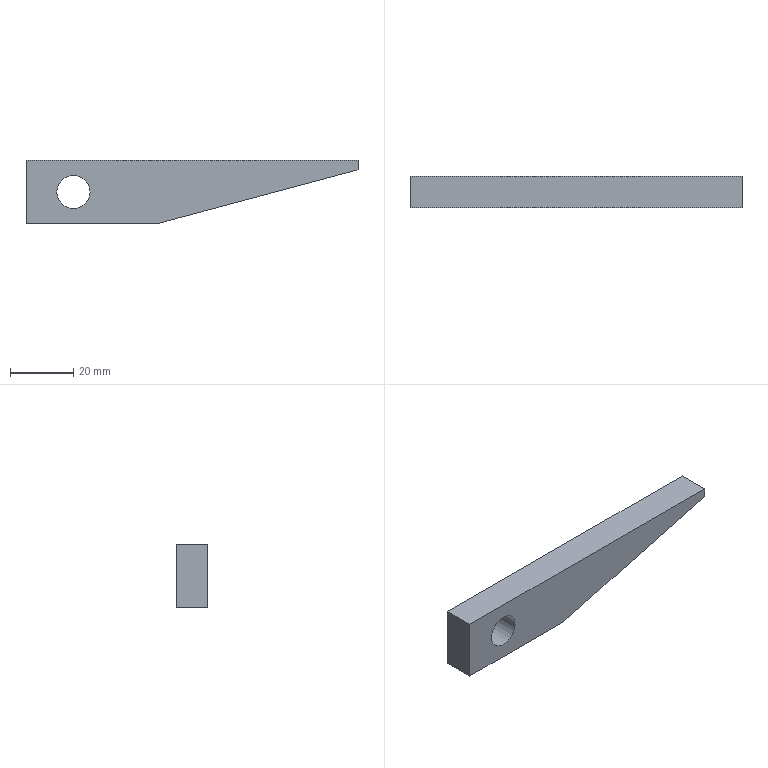Part | NX | features solid 2 | 1 solid | 8 faces | box 105 x 10 x 20 mm | volume 14741 mm3 | plane 7 | cylinder 1 | commonest cylinder face diameters 10.5 x1
STEP:
#1=CARTESIAN_POINT('',(-925.,90.,-134.));
#2=VERTEX_POINT('',#1);
#3=CARTESIAN_POINT('',(-883.445,90.,-134.));
#4=VERTEX_POINT('',#3);
#5=CARTESIAN_POINT('',(-925.,90.,-134.));
#6=DIRECTION('',(1.,0.,0.));
#7=VECTOR('',#6,1000.);
#8=LINE('',#5,#7);
#9=EDGE_CURVE('',#2,#4,#8,.T.);
#10=ORIENTED_EDGE('',*,*,#9,.T.);
#11=CARTESIAN_POINT('',(-883.445,80.,-134.));
#12=VERTEX_POINT('',#11);
#13=CARTESIAN_POINT('',(-883.445,90.,-134.));
#14=DIRECTION('',(0.,-1.,0.));
#15=VECTOR('',#14,1000.);
#16=LINE('',#13,#15);
#17=EDGE_CURVE('',#4,#12,#16,.T.);
#18=ORIENTED_EDGE('',*,*,#17,.T.);
#19=CARTESIAN_POINT('',(-925.,80.,-134.));
#20=VERTEX_POINT('',#19);
#21=CARTESIAN_POINT('',(-925.,80.,-134.));
#22=DIRECTION('',(1.,0.,0.));
#23=VECTOR('',#22,1000.);
#24=LINE('',#21,#23);
#25=EDGE_CURVE('',#20,#12,#24,.T.);
#26=ORIENTED_EDGE('',*,*,#25,.F.);
#27=CARTESIAN_POINT('',(-925.,90.,-134.));
#28=DIRECTION('',(0.,-1.,0.));
#29=VECTOR('',#28,1000.);
#30=LINE('',#27,#29);
#31=EDGE_CURVE('',#2,#20,#30,.T.);
#32=ORIENTED_EDGE('',*,*,#31,.F.);
#33=EDGE_LOOP('',(#10,#18,#26,#32));
#34=FACE_BOUND('',#33,.T.);
#35=CARTESIAN_POINT('',(-925.,90.,-134.));
#36=DIRECTION('',(0.,0.,-1.));
#37=DIRECTION('',(-1.,0.,0.));
#38=AXIS2_PLACEMENT_3D('',#35,#36,#37);
#39=PLANE('',#38);
#40=ADVANCED_FACE('',(#34),#39,.T.);
#41=CARTESIAN_POINT('',(-820.,80.,-117.));
#42=VERTEX_POINT('',#41);
#43=CARTESIAN_POINT('',(-820.,80.,-114.));
#44=VERTEX_POINT('',#43);
#45=CARTESIAN_POINT('',(-820.,80.,-134.));
#46=DIRECTION('',(0.,0.,1.));
#47=VECTOR('',#46,1000.);
#48=LINE('',#45,#47);
#49=EDGE_CURVE('',#42,#44,#48,.T.);
#50=ORIENTED_EDGE('',*,*,#49,.F.);
#51=CARTESIAN_POINT('',(-820.,90.,-117.));
#52=VERTEX_POINT('',#51);
#53=CARTESIAN_POINT('',(-820.,90.,-117.));
#54=DIRECTION('',(0.,1.,0.));
#55=VECTOR('',#54,1000.);
#56=LINE('',#53,#55);
#57=EDGE_CURVE('',#42,#52,#56,.T.);
#58=ORIENTED_EDGE('',*,*,#57,.T.);
#59=CARTESIAN_POINT('',(-820.,90.,-114.));
#60=VERTEX_POINT('',#59);
#61=CARTESIAN_POINT('',(-820.,90.,-134.));
#62=DIRECTION('',(0.,0.,1.));
#63=VECTOR('',#62,1000.);
#64=LINE('',#61,#63);
#65=EDGE_CURVE('',#52,#60,#64,.T.);
#66=ORIENTED_EDGE('',*,*,#65,.T.);
#67=CARTESIAN_POINT('',(-820.,90.,-114.));
#68=DIRECTION('',(0.,-1.,0.));
#69=VECTOR('',#68,1000.);
#70=LINE('',#67,#69);
#71=EDGE_CURVE('',#60,#44,#70,.T.);
#72=ORIENTED_EDGE('',*,*,#71,.T.);
#73=EDGE_LOOP('',(#50,#58,#66,#72));
#74=FACE_BOUND('',#73,.T.);
#75=CARTESIAN_POINT('',(-820.,90.,-134.));
#76=DIRECTION('',(1.,0.,0.));
#77=DIRECTION('',(0.,0.,-1.));
#78=AXIS2_PLACEMENT_3D('',#75,#76,#77);
#79=PLANE('',#78);
#80=ADVANCED_FACE('',(#74),#79,.T.);
#81=CARTESIAN_POINT('',(-925.,80.,-114.));
#82=VERTEX_POINT('',#81);
#83=CARTESIAN_POINT('',(-820.,80.,-114.));
#84=DIRECTION('',(-1.,0.,0.));
#85=VECTOR('',#84,1000.);
#86=LINE('',#83,#85);
#87=EDGE_CURVE('',#44,#82,#86,.T.);
#88=ORIENTED_EDGE('',*,*,#87,.F.);
#89=ORIENTED_EDGE('',*,*,#71,.F.);
#90=CARTESIAN_POINT('',(-925.,90.,-114.));
#91=VERTEX_POINT('',#90);
#92=CARTESIAN_POINT('',(-820.,90.,-114.));
#93=DIRECTION('',(-1.,0.,0.));
#94=VECTOR('',#93,1000.);
#95=LINE('',#92,#94);
#96=EDGE_CURVE('',#60,#91,#95,.T.);
#97=ORIENTED_EDGE('',*,*,#96,.T.);
#98=CARTESIAN_POINT('',(-925.,90.,-114.));
#99=DIRECTION('',(0.,-1.,0.));
#100=VECTOR('',#99,1000.);
#101=LINE('',#98,#100);
#102=EDGE_CURVE('',#91,#82,#101,.T.);
#103=ORIENTED_EDGE('',*,*,#102,.T.);
#104=EDGE_LOOP('',(#88,#89,#97,#103));
#105=FACE_BOUND('',#104,.T.);
#106=CARTESIAN_POINT('',(-820.,90.,-114.));
#107=DIRECTION('',(0.,0.,1.));
#108=DIRECTION('',(0.,1.,0.));
#109=AXIS2_PLACEMENT_3D('',#106,#107,#108);
#110=PLANE('',#109);
#111=ADVANCED_FACE('',(#105),#110,.T.);
#112=CARTESIAN_POINT('',(-925.,80.,-114.));
#113=DIRECTION('',(0.,0.,-1.));
#114=VECTOR('',#113,1000.);
#115=LINE('',#112,#114);
#116=EDGE_CURVE('',#82,#20,#115,.T.);
#117=ORIENTED_EDGE('',*,*,#116,.F.);
#118=ORIENTED_EDGE('',*,*,#102,.F.);
#119=CARTESIAN_POINT('',(-925.,90.,-114.));
#120=DIRECTION('',(0.,0.,-1.));
#121=VECTOR('',#120,1000.);
#122=LINE('',#119,#121);
#123=EDGE_CURVE('',#91,#2,#122,.T.);
#124=ORIENTED_EDGE('',*,*,#123,.T.);
#125=ORIENTED_EDGE('',*,*,#31,.T.);
#126=EDGE_LOOP('',(#117,#118,#124,#125));
#127=FACE_BOUND('',#126,.T.);
#128=CARTESIAN_POINT('',(-925.,90.,-114.));
#129=DIRECTION('',(-1.,0.,0.));
#130=DIRECTION('',(0.,0.,1.));
#131=AXIS2_PLACEMENT_3D('',#128,#129,#130);
#132=PLANE('',#131);
#133=ADVANCED_FACE('',(#127),#132,.T.);
#134=CARTESIAN_POINT('',(-915.25,90.,-124.));
#135=VERTEX_POINT('',#134);
#136=CARTESIAN_POINT('',(-910.,90.,-124.));
#137=DIRECTION('',(0.,1.,0.));
#138=DIRECTION('',(-1.,0.,0.));
#139=AXIS2_PLACEMENT_3D('',#136,#137,#138);
#140=CIRCLE('',#139,5.25);
#141=EDGE_CURVE('',#135,#135,#140,.T.);
#142=ORIENTED_EDGE('',*,*,#141,.T.);
#143=EDGE_LOOP('',(#142));
#144=FACE_BOUND('',#143,.T.);
#145=CARTESIAN_POINT('',(-915.25,80.,-124.));
#146=VERTEX_POINT('',#145);
#147=CARTESIAN_POINT('',(-910.,80.,-124.));
#148=DIRECTION('',(0.,1.,0.));
#149=DIRECTION('',(-1.,0.,0.));
#150=AXIS2_PLACEMENT_3D('',#147,#148,#149);
#151=CIRCLE('',#150,5.25);
#152=EDGE_CURVE('',#146,#146,#151,.T.);
#153=ORIENTED_EDGE('',*,*,#152,.F.);
#154=EDGE_LOOP('',(#153));
#155=FACE_BOUND('',#154,.T.);
#156=CARTESIAN_POINT('',(-910.,90.,-124.));
#157=DIRECTION('',(0.,-1.,0.));
#158=DIRECTION('',(0.,0.,1.));
#159=AXIS2_PLACEMENT_3D('',#156,#157,#158);
#160=CYLINDRICAL_SURFACE('',#159,5.25);
#161=ADVANCED_FACE('',(#144,#155),#160,.F.);
#162=ORIENTED_EDGE('',*,*,#65,.F.);
#163=CARTESIAN_POINT('',(-883.445,90.,-134.));
#164=DIRECTION('',(0.9659,0.,0.2588));
#165=VECTOR('',#164,1000.);
#166=LINE('',#163,#165);
#167=EDGE_CURVE('',#52,#4,#166,.F.);
#168=ORIENTED_EDGE('',*,*,#167,.T.);
#169=ORIENTED_EDGE('',*,*,#9,.F.);
#170=ORIENTED_EDGE('',*,*,#123,.F.);
#171=ORIENTED_EDGE('',*,*,#96,.F.);
#172=EDGE_LOOP('',(#162,#168,#169,#170,#171));
#173=FACE_BOUND('',#172,.T.);
#174=ORIENTED_EDGE('',*,*,#141,.F.);
#175=EDGE_LOOP('',(#174));
#176=FACE_BOUND('',#175,.T.);
#177=CARTESIAN_POINT('',(-820.,90.,-134.));
#178=DIRECTION('',(0.,-1.,0.));
#179=DIRECTION('',(0.,0.,1.));
#180=AXIS2_PLACEMENT_3D('',#177,#178,#179);
#181=PLANE('',#180);
#182=ADVANCED_FACE('',(#173,#176),#181,.F.);
#183=ORIENTED_EDGE('',*,*,#25,.T.);
#184=CARTESIAN_POINT('',(-824.25,80.,-118.139));
#185=DIRECTION('',(-0.9659,0.,-0.2588));
#186=VECTOR('',#185,1000.);
#187=LINE('',#184,#186);
#188=EDGE_CURVE('',#12,#42,#187,.F.);
#189=ORIENTED_EDGE('',*,*,#188,.T.);
#190=ORIENTED_EDGE('',*,*,#49,.T.);
#191=ORIENTED_EDGE('',*,*,#87,.T.);
#192=ORIENTED_EDGE('',*,*,#116,.T.);
#193=EDGE_LOOP('',(#183,#189,#190,#191,#192));
#194=FACE_BOUND('',#193,.T.);
#195=ORIENTED_EDGE('',*,*,#152,.T.);
#196=EDGE_LOOP('',(#195));
#197=FACE_BOUND('',#196,.T.);
#198=CARTESIAN_POINT('',(-820.,80.,-134.));
#199=DIRECTION('',(0.,-1.,0.));
#200=DIRECTION('',(0.,0.,1.));
#201=AXIS2_PLACEMENT_3D('',#198,#199,#200);
#202=PLANE('',#201);
#203=ADVANCED_FACE('',(#194,#197),#202,.T.);
#204=ORIENTED_EDGE('',*,*,#167,.F.);
#205=ORIENTED_EDGE('',*,*,#57,.F.);
#206=ORIENTED_EDGE('',*,*,#188,.F.);
#207=ORIENTED_EDGE('',*,*,#17,.F.);
#208=EDGE_LOOP('',(#204,#205,#206,#207));
#209=FACE_BOUND('',#208,.T.);
#210=CARTESIAN_POINT('',(-883.445,90.,-134.));
#211=DIRECTION('',(-0.2588,0.,0.9659));
#212=DIRECTION('',(0.9659,0.,0.2588));
#213=AXIS2_PLACEMENT_3D('',#210,#211,#212);
#214=PLANE('',#213);
#215=ADVANCED_FACE('',(#209),#214,.F.);
#216=CLOSED_SHELL('',(#40,#80,#111,#133,#161,#182,#203,#215));
#217=MANIFOLD_SOLID_BREP('',#216);
#218=(LENGTH_UNIT()NAMED_UNIT(*)SI_UNIT(.MILLI.,.METRE.));
#219=UNCERTAINTY_MEASURE_WITH_UNIT(LENGTH_MEASURE(0.00001),#218,'','');
#220=(NAMED_UNIT(*)PLANE_ANGLE_UNIT()SI_UNIT($,.RADIAN.));
#221=(NAMED_UNIT(*)SI_UNIT($,.STERADIAN.)SOLID_ANGLE_UNIT());
#222=(GEOMETRIC_REPRESENTATION_CONTEXT(3)GLOBAL_UNCERTAINTY_ASSIGNED_CONTEXT((#219))GLOBAL_UNIT_ASSIGNED_CONTEXT((#218,#220,#221))REPRESENTATION_CONTEXT('',''));
#223=ADVANCED_BREP_SHAPE_REPRESENTATION('',(#217),#222);